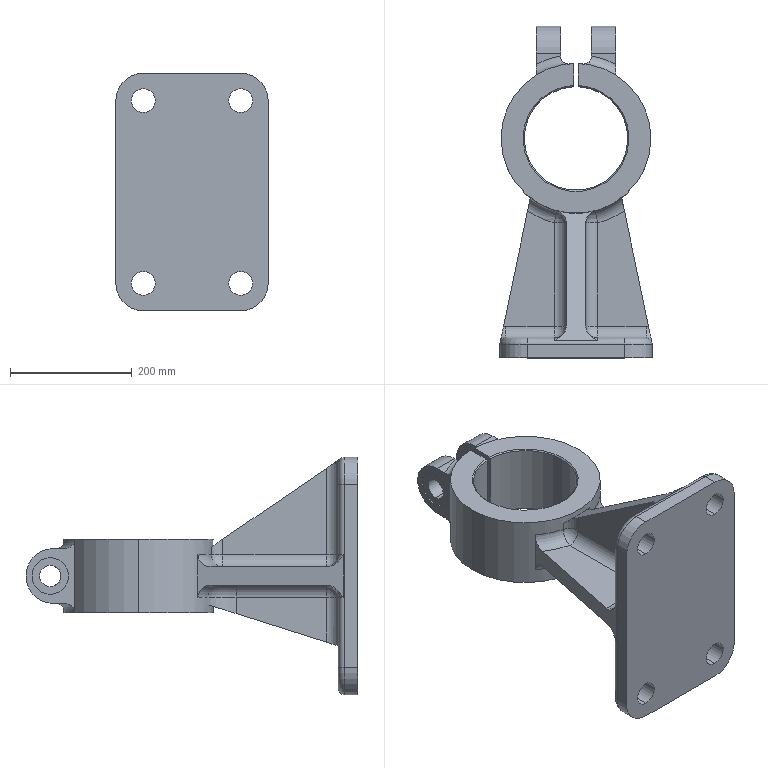Part | SolidWorks | features ICE 9, Fillet 7, Chamfer 1, Extrusion 1, LPattern 1 | 1 solid | 130 faces | box 250 x 545 x 390 mm | volume 8795912 mm3 | cylinder 58 | plane 40 | torus 20 | cone 6 | sphere 6 | commonest cylinder face diameters 40 x14 39 x8 70 x8 20 x6 90 x6 35 x4